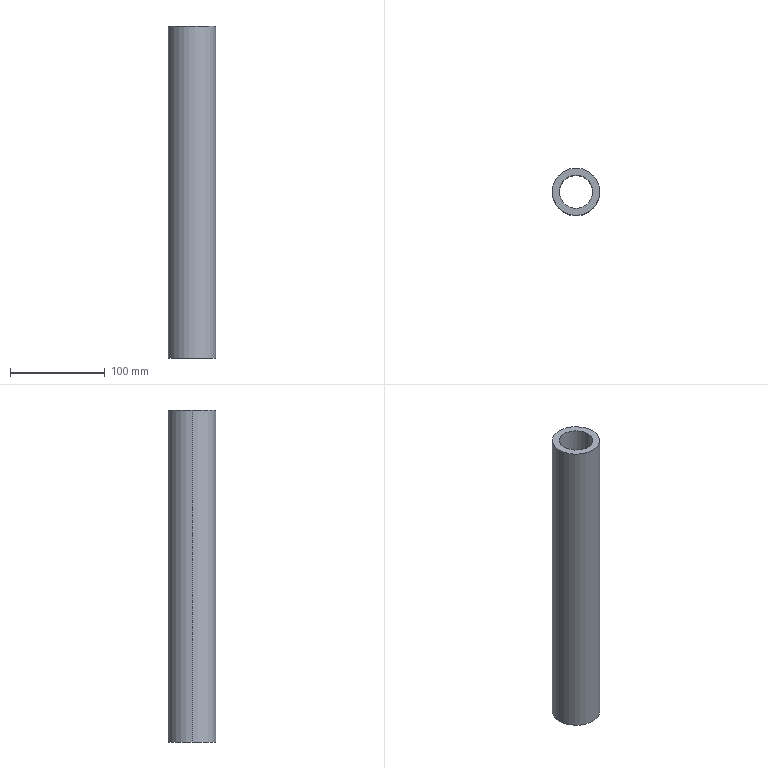Part | STEP file | mounting assembly column ZCD06-D50-L350 | 1 solid | 6 faces | box 50 x 50 x 350 mm | volume 350484 mm3 | cylinder 4 | plane 2 | commonest cylinder face diameters 35 x2 50 x2
STEP:
#1=CARTESIAN_POINT('',(0.,0.,0.));
#2=DIRECTION('',(0.,0.,1.));
#3=DIRECTION('',(1.,0.,0.));
#4=AXIS2_PLACEMENT_3D('',#1,#2,#3);
#5=CARTESIAN_POINT('',(25.,0.,0.));
#6=VERTEX_POINT('',#5);
#7=CARTESIAN_POINT('',(-25.,0.,0.));
#8=VERTEX_POINT('',#7);
#9=CARTESIAN_POINT('',(0.,0.,0.));
#10=DIRECTION('',(0.,0.,1.));
#11=DIRECTION('',(1.,0.,0.));
#12=AXIS2_PLACEMENT_3D('',#9,#10,#11);
#13=CIRCLE('',#12,25.);
#14=CARTESIAN_POINT('',(0.,0.,460.));
#15=DIRECTION('',(0.,0.,1.));
#16=DIRECTION('',(1.,0.,0.));
#17=AXIS2_PLACEMENT_3D('',#14,#15,#16);
#18=CYLINDRICAL_SURFACE('',#17,25.);
#19=CARTESIAN_POINT('',(0.,-460.));
#20=DIRECTION('',(1.,0.));
#21=VECTOR('',#20,1.);
#22=LINE('',#19,#21);
#23=(GEOMETRIC_REPRESENTATION_CONTEXT(2)PARAMETRIC_REPRESENTATION_CONTEXT()REPRESENTATION_CONTEXT('',''));
#24=DEFINITIONAL_REPRESENTATION('',(#22),#23);
#25=PCURVE('',#18,#24);
#26=CARTESIAN_POINT('',(0.,0.,0.));
#27=DIRECTION('',(0.,0.,1.));
#28=DIRECTION('',(1.,0.,0.));
#29=AXIS2_PLACEMENT_3D('',#26,#27,#28);
#30=PLANE('',#29);
#31=CARTESIAN_POINT('',(0.,0.));
#32=DIRECTION('',(1.,0.));
#33=AXIS2_PLACEMENT_2D('',#31,#32);
#34=CIRCLE('',#33,25.);
#35=(GEOMETRIC_REPRESENTATION_CONTEXT(2)PARAMETRIC_REPRESENTATION_CONTEXT()REPRESENTATION_CONTEXT('',''));
#36=DEFINITIONAL_REPRESENTATION('',(#34),#35);
#37=PCURVE('',#30,#36);
#38=SURFACE_CURVE('',#13,(#25,#37),.PCURVE_S1.);
#39=EDGE_CURVE('',#6,#8,#38,.T.);
#40=ORIENTED_EDGE('',*,*,#39,.T.);
#41=CARTESIAN_POINT('',(-25.,0.,350.));
#42=VERTEX_POINT('',#41);
#43=CARTESIAN_POINT('',(-25.,0.,460.));
#44=DIRECTION('',(0.,0.,1.));
#45=VECTOR('',#44,1.);
#46=LINE('',#43,#45);
#47=CARTESIAN_POINT('',(3.142,0.));
#48=DIRECTION('',(0.,1.));
#49=VECTOR('',#48,1.);
#50=LINE('',#47,#49);
#51=(GEOMETRIC_REPRESENTATION_CONTEXT(2)PARAMETRIC_REPRESENTATION_CONTEXT()REPRESENTATION_CONTEXT('',''));
#52=DEFINITIONAL_REPRESENTATION('',(#50),#51);
#53=PCURVE('',#18,#52);
#54=CARTESIAN_POINT('',(0.,0.,460.));
#55=DIRECTION('',(0.,0.,1.));
#56=DIRECTION('',(1.,0.,0.));
#57=AXIS2_PLACEMENT_3D('',#54,#55,#56);
#58=CYLINDRICAL_SURFACE('',#57,25.);
#59=CARTESIAN_POINT('',(3.142,0.));
#60=DIRECTION('',(0.,1.));
#61=VECTOR('',#60,1.);
#62=LINE('',#59,#61);
#63=(GEOMETRIC_REPRESENTATION_CONTEXT(2)PARAMETRIC_REPRESENTATION_CONTEXT()REPRESENTATION_CONTEXT('',''));
#64=DEFINITIONAL_REPRESENTATION('',(#62),#63);
#65=PCURVE('',#58,#64);
#66=SURFACE_CURVE('',#46,(#53,#65),.PCURVE_S1.);
#67=EDGE_CURVE('',#8,#42,#66,.T.);
#68=ORIENTED_EDGE('',*,*,#67,.T.);
#69=CARTESIAN_POINT('',(25.,0.,350.));
#70=VERTEX_POINT('',#69);
#71=CARTESIAN_POINT('',(0.,0.,350.));
#72=DIRECTION('',(0.,0.,1.));
#73=DIRECTION('',(1.,0.,0.));
#74=AXIS2_PLACEMENT_3D('',#71,#72,#73);
#75=CIRCLE('',#74,25.);
#76=CARTESIAN_POINT('',(0.,-110.));
#77=DIRECTION('',(1.,0.));
#78=VECTOR('',#77,1.);
#79=LINE('',#76,#78);
#80=(GEOMETRIC_REPRESENTATION_CONTEXT(2)PARAMETRIC_REPRESENTATION_CONTEXT()REPRESENTATION_CONTEXT('',''));
#81=DEFINITIONAL_REPRESENTATION('',(#79),#80);
#82=PCURVE('',#18,#81);
#83=CARTESIAN_POINT('',(0.,0.,350.));
#84=DIRECTION('',(0.,0.,1.));
#85=DIRECTION('',(1.,0.,0.));
#86=AXIS2_PLACEMENT_3D('',#83,#84,#85);
#87=PLANE('',#86);
#88=CARTESIAN_POINT('',(0.,0.));
#89=DIRECTION('',(1.,0.));
#90=AXIS2_PLACEMENT_2D('',#88,#89);
#91=CIRCLE('',#90,25.);
#92=(GEOMETRIC_REPRESENTATION_CONTEXT(2)PARAMETRIC_REPRESENTATION_CONTEXT()REPRESENTATION_CONTEXT('',''));
#93=DEFINITIONAL_REPRESENTATION('',(#91),#92);
#94=PCURVE('',#87,#93);
#95=SURFACE_CURVE('',#75,(#82,#94),.PCURVE_S1.);
#96=EDGE_CURVE('',#70,#42,#95,.T.);
#97=ORIENTED_EDGE('',*,*,#96,.F.);
#98=CARTESIAN_POINT('',(25.,0.,460.));
#99=DIRECTION('',(0.,0.,1.));
#100=VECTOR('',#99,1.);
#101=LINE('',#98,#100);
#102=CARTESIAN_POINT('',(0.,0.));
#103=DIRECTION('',(0.,1.));
#104=VECTOR('',#103,1.);
#105=LINE('',#102,#104);
#106=(GEOMETRIC_REPRESENTATION_CONTEXT(2)PARAMETRIC_REPRESENTATION_CONTEXT()REPRESENTATION_CONTEXT('',''));
#107=DEFINITIONAL_REPRESENTATION('',(#105),#106);
#108=PCURVE('',#18,#107);
#109=CARTESIAN_POINT('',(6.283,0.));
#110=DIRECTION('',(0.,1.));
#111=VECTOR('',#110,1.);
#112=LINE('',#109,#111);
#113=(GEOMETRIC_REPRESENTATION_CONTEXT(2)PARAMETRIC_REPRESENTATION_CONTEXT()REPRESENTATION_CONTEXT('',''));
#114=DEFINITIONAL_REPRESENTATION('',(#112),#113);
#115=PCURVE('',#58,#114);
#116=SURFACE_CURVE('',#101,(#108,#115),.PCURVE_S1.);
#117=EDGE_CURVE('',#6,#70,#116,.T.);
#118=ORIENTED_EDGE('',*,*,#117,.F.);
#119=EDGE_LOOP('',(#40,#68,#97,#118));
#120=FACE_BOUND('',#119,.T.);
#121=ADVANCED_FACE('',(#120),#18,.T.);
#122=CARTESIAN_POINT('',(17.5,0.,0.));
#123=VERTEX_POINT('',#122);
#124=CARTESIAN_POINT('',(17.5,0.,350.));
#125=VERTEX_POINT('',#124);
#126=CARTESIAN_POINT('',(17.5,0.,460.));
#127=DIRECTION('',(0.,0.,1.));
#128=VECTOR('',#127,1.);
#129=LINE('',#126,#128);
#130=CARTESIAN_POINT('',(0.,0.,460.));
#131=DIRECTION('',(0.,0.,1.));
#132=DIRECTION('',(1.,0.,0.));
#133=AXIS2_PLACEMENT_3D('',#130,#131,#132);
#134=CYLINDRICAL_SURFACE('',#133,17.5);
#135=CARTESIAN_POINT('',(6.283,0.));
#136=DIRECTION('',(0.,1.));
#137=VECTOR('',#136,1.);
#138=LINE('',#135,#137);
#139=(GEOMETRIC_REPRESENTATION_CONTEXT(2)PARAMETRIC_REPRESENTATION_CONTEXT()REPRESENTATION_CONTEXT('',''));
#140=DEFINITIONAL_REPRESENTATION('',(#138),#139);
#141=PCURVE('',#134,#140);
#142=CARTESIAN_POINT('',(0.,0.,460.));
#143=DIRECTION('',(0.,0.,1.));
#144=DIRECTION('',(1.,0.,0.));
#145=AXIS2_PLACEMENT_3D('',#142,#143,#144);
#146=CYLINDRICAL_SURFACE('',#145,17.5);
#147=CARTESIAN_POINT('',(0.,0.));
#148=DIRECTION('',(0.,1.));
#149=VECTOR('',#148,1.);
#150=LINE('',#147,#149);
#151=(GEOMETRIC_REPRESENTATION_CONTEXT(2)PARAMETRIC_REPRESENTATION_CONTEXT()REPRESENTATION_CONTEXT('',''));
#152=DEFINITIONAL_REPRESENTATION('',(#150),#151);
#153=PCURVE('',#146,#152);
#154=SURFACE_CURVE('',#129,(#141,#153),.PCURVE_S1.);
#155=EDGE_CURVE('',#123,#125,#154,.T.);
#156=ORIENTED_EDGE('',*,*,#155,.T.);
#157=CARTESIAN_POINT('',(-17.5,0.,350.));
#158=VERTEX_POINT('',#157);
#159=CARTESIAN_POINT('',(0.,0.,350.));
#160=DIRECTION('',(0.,0.,1.));
#161=DIRECTION('',(1.,0.,0.));
#162=AXIS2_PLACEMENT_3D('',#159,#160,#161);
#163=CIRCLE('',#162,17.5);
#164=CARTESIAN_POINT('',(0.,-110.));
#165=DIRECTION('',(1.,0.));
#166=VECTOR('',#165,1.);
#167=LINE('',#164,#166);
#168=(GEOMETRIC_REPRESENTATION_CONTEXT(2)PARAMETRIC_REPRESENTATION_CONTEXT()REPRESENTATION_CONTEXT('',''));
#169=DEFINITIONAL_REPRESENTATION('',(#167),#168);
#170=PCURVE('',#134,#169);
#171=CARTESIAN_POINT('',(0.,0.));
#172=DIRECTION('',(1.,0.));
#173=AXIS2_PLACEMENT_2D('',#171,#172);
#174=CIRCLE('',#173,17.5);
#175=(GEOMETRIC_REPRESENTATION_CONTEXT(2)PARAMETRIC_REPRESENTATION_CONTEXT()REPRESENTATION_CONTEXT('',''));
#176=DEFINITIONAL_REPRESENTATION('',(#174),#175);
#177=PCURVE('',#87,#176);
#178=SURFACE_CURVE('',#163,(#170,#177),.PCURVE_S1.);
#179=EDGE_CURVE('',#158,#125,#178,.T.);
#180=ORIENTED_EDGE('',*,*,#179,.F.);
#181=CARTESIAN_POINT('',(-17.5,0.,0.));
#182=VERTEX_POINT('',#181);
#183=CARTESIAN_POINT('',(-17.5,0.,460.));
#184=DIRECTION('',(0.,0.,1.));
#185=VECTOR('',#184,1.);
#186=LINE('',#183,#185);
#187=CARTESIAN_POINT('',(3.142,0.));
#188=DIRECTION('',(0.,1.));
#189=VECTOR('',#188,1.);
#190=LINE('',#187,#189);
#191=(GEOMETRIC_REPRESENTATION_CONTEXT(2)PARAMETRIC_REPRESENTATION_CONTEXT()REPRESENTATION_CONTEXT('',''));
#192=DEFINITIONAL_REPRESENTATION('',(#190),#191);
#193=PCURVE('',#134,#192);
#194=CARTESIAN_POINT('',(3.142,0.));
#195=DIRECTION('',(0.,1.));
#196=VECTOR('',#195,1.);
#197=LINE('',#194,#196);
#198=(GEOMETRIC_REPRESENTATION_CONTEXT(2)PARAMETRIC_REPRESENTATION_CONTEXT()REPRESENTATION_CONTEXT('',''));
#199=DEFINITIONAL_REPRESENTATION('',(#197),#198);
#200=PCURVE('',#146,#199);
#201=SURFACE_CURVE('',#186,(#193,#200),.PCURVE_S1.);
#202=EDGE_CURVE('',#182,#158,#201,.T.);
#203=ORIENTED_EDGE('',*,*,#202,.F.);
#204=CARTESIAN_POINT('',(0.,0.,0.));
#205=DIRECTION('',(0.,0.,-1.));
#206=DIRECTION('',(1.,0.,0.));
#207=AXIS2_PLACEMENT_3D('',#204,#205,#206);
#208=CIRCLE('',#207,17.5);
#209=CARTESIAN_POINT('',(6.283,-460.));
#210=DIRECTION('',(-1.,0.));
#211=VECTOR('',#210,1.);
#212=LINE('',#209,#211);
#213=(GEOMETRIC_REPRESENTATION_CONTEXT(2)PARAMETRIC_REPRESENTATION_CONTEXT()REPRESENTATION_CONTEXT('',''));
#214=DEFINITIONAL_REPRESENTATION('',(#212),#213);
#215=PCURVE('',#134,#214);
#216=CARTESIAN_POINT('',(17.5,0.));
#217=CARTESIAN_POINT('',(17.5,-30.311));
#218=CARTESIAN_POINT('',(-8.75,-15.155));
#219=CARTESIAN_POINT('',(-35.,0.));
#220=CARTESIAN_POINT('',(-8.75,15.155));
#221=CARTESIAN_POINT('',(17.5,30.311));
#222=CARTESIAN_POINT('',(17.5,0.));
#223=(BOUNDED_CURVE()B_SPLINE_CURVE(2,(#216,#217,#218,#219,#220,#221,#222),.UNSPECIFIED.,.T.,.F.)B_SPLINE_CURVE_WITH_KNOTS((1,2,2,2,2,1),(-2.094,0.,2.094,4.189,6.283,8.378),.UNSPECIFIED.)CURVE()GEOMETRIC_REPRESENTATION_ITEM()RATIONAL_B_SPLINE_CURVE((1.,0.5,1.,0.5,1.,0.5,1.))REPRESENTATION_ITEM(''));
#224=(GEOMETRIC_REPRESENTATION_CONTEXT(2)PARAMETRIC_REPRESENTATION_CONTEXT()REPRESENTATION_CONTEXT('',''));
#225=DEFINITIONAL_REPRESENTATION('',(#223),#224);
#226=PCURVE('',#30,#225);
#227=SURFACE_CURVE('',#208,(#215,#226),.PCURVE_S1.);
#228=EDGE_CURVE('',#123,#182,#227,.T.);
#229=ORIENTED_EDGE('',*,*,#228,.F.);
#230=EDGE_LOOP('',(#156,#180,#203,#229));
#231=FACE_BOUND('',#230,.F.);
#232=ADVANCED_FACE('',(#231),#134,.F.);
#233=ORIENTED_EDGE('',*,*,#67,.F.);
#234=CARTESIAN_POINT('',(0.,0.,0.));
#235=DIRECTION('',(0.,0.,1.));
#236=DIRECTION('',(1.,0.,0.));
#237=AXIS2_PLACEMENT_3D('',#234,#235,#236);
#238=CIRCLE('',#237,25.);
#239=CARTESIAN_POINT('',(0.,-460.));
#240=DIRECTION('',(1.,0.));
#241=VECTOR('',#240,1.);
#242=LINE('',#239,#241);
#243=(GEOMETRIC_REPRESENTATION_CONTEXT(2)PARAMETRIC_REPRESENTATION_CONTEXT()REPRESENTATION_CONTEXT('',''));
#244=DEFINITIONAL_REPRESENTATION('',(#242),#243);
#245=PCURVE('',#58,#244);
#246=CARTESIAN_POINT('',(0.,0.));
#247=DIRECTION('',(1.,0.));
#248=AXIS2_PLACEMENT_2D('',#246,#247);
#249=CIRCLE('',#248,25.);
#250=(GEOMETRIC_REPRESENTATION_CONTEXT(2)PARAMETRIC_REPRESENTATION_CONTEXT()REPRESENTATION_CONTEXT('',''));
#251=DEFINITIONAL_REPRESENTATION('',(#249),#250);
#252=PCURVE('',#30,#251);
#253=SURFACE_CURVE('',#238,(#245,#252),.PCURVE_S1.);
#254=EDGE_CURVE('',#8,#6,#253,.T.);
#255=ORIENTED_EDGE('',*,*,#254,.T.);
#256=ORIENTED_EDGE('',*,*,#117,.T.);
#257=CARTESIAN_POINT('',(0.,0.,350.));
#258=DIRECTION('',(0.,0.,1.));
#259=DIRECTION('',(1.,0.,0.));
#260=AXIS2_PLACEMENT_3D('',#257,#258,#259);
#261=CIRCLE('',#260,25.);
#262=CARTESIAN_POINT('',(0.,-110.));
#263=DIRECTION('',(1.,0.));
#264=VECTOR('',#263,1.);
#265=LINE('',#262,#264);
#266=(GEOMETRIC_REPRESENTATION_CONTEXT(2)PARAMETRIC_REPRESENTATION_CONTEXT()REPRESENTATION_CONTEXT('',''));
#267=DEFINITIONAL_REPRESENTATION('',(#265),#266);
#268=PCURVE('',#58,#267);
#269=CARTESIAN_POINT('',(0.,0.));
#270=DIRECTION('',(1.,0.));
#271=AXIS2_PLACEMENT_2D('',#269,#270);
#272=CIRCLE('',#271,25.);
#273=(GEOMETRIC_REPRESENTATION_CONTEXT(2)PARAMETRIC_REPRESENTATION_CONTEXT()REPRESENTATION_CONTEXT('',''));
#274=DEFINITIONAL_REPRESENTATION('',(#272),#273);
#275=PCURVE('',#87,#274);
#276=SURFACE_CURVE('',#261,(#268,#275),.PCURVE_S1.);
#277=EDGE_CURVE('',#42,#70,#276,.T.);
#278=ORIENTED_EDGE('',*,*,#277,.F.);
#279=EDGE_LOOP('',(#233,#255,#256,#278));
#280=FACE_BOUND('',#279,.T.);
#281=ADVANCED_FACE('',(#280),#58,.T.);
#282=ORIENTED_EDGE('',*,*,#39,.F.);
#283=ORIENTED_EDGE('',*,*,#254,.F.);
#284=EDGE_LOOP('',(#282,#283));
#285=FACE_BOUND('',#284,.T.);
#286=ORIENTED_EDGE('',*,*,#228,.F.);
#287=CARTESIAN_POINT('',(0.,0.,0.));
#288=DIRECTION('',(0.,0.,-1.));
#289=DIRECTION('',(1.,0.,0.));
#290=AXIS2_PLACEMENT_3D('',#287,#288,#289);
#291=CIRCLE('',#290,17.5);
#292=CARTESIAN_POINT('',(17.5,0.));
#293=CARTESIAN_POINT('',(17.5,-30.311));
#294=CARTESIAN_POINT('',(-8.75,-15.155));
#295=CARTESIAN_POINT('',(-35.,0.));
#296=CARTESIAN_POINT('',(-8.75,15.155));
#297=CARTESIAN_POINT('',(17.5,30.311));
#298=CARTESIAN_POINT('',(17.5,0.));
#299=(BOUNDED_CURVE()B_SPLINE_CURVE(2,(#292,#293,#294,#295,#296,#297,#298),.UNSPECIFIED.,.T.,.F.)B_SPLINE_CURVE_WITH_KNOTS((1,2,2,2,2,1),(-2.094,0.,2.094,4.189,6.283,8.378),.UNSPECIFIED.)CURVE()GEOMETRIC_REPRESENTATION_ITEM()RATIONAL_B_SPLINE_CURVE((1.,0.5,1.,0.5,1.,0.5,1.))REPRESENTATION_ITEM(''));
#300=(GEOMETRIC_REPRESENTATION_CONTEXT(2)PARAMETRIC_REPRESENTATION_CONTEXT()REPRESENTATION_CONTEXT('',''));
#301=DEFINITIONAL_REPRESENTATION('',(#299),#300);
#302=PCURVE('',#30,#301);
#303=CARTESIAN_POINT('',(6.283,-460.));
#304=DIRECTION('',(-1.,0.));
#305=VECTOR('',#304,1.);
#306=LINE('',#303,#305);
#307=(GEOMETRIC_REPRESENTATION_CONTEXT(2)PARAMETRIC_REPRESENTATION_CONTEXT()REPRESENTATION_CONTEXT('',''));
#308=DEFINITIONAL_REPRESENTATION('',(#306),#307);
#309=PCURVE('',#146,#308);
#310=SURFACE_CURVE('',#291,(#302,#309),.PCURVE_S1.);
#311=EDGE_CURVE('',#182,#123,#310,.T.);
#312=ORIENTED_EDGE('',*,*,#311,.F.);
#313=EDGE_LOOP('',(#286,#312));
#314=FACE_BOUND('',#313,.T.);
#315=ADVANCED_FACE('',(#285,#314),#30,.F.);
#316=CARTESIAN_POINT('',(0.,0.,350.));
#317=DIRECTION('',(0.,0.,1.));
#318=DIRECTION('',(1.,0.,0.));
#319=AXIS2_PLACEMENT_3D('',#316,#317,#318);
#320=CIRCLE('',#319,17.5);
#321=CARTESIAN_POINT('',(0.,-110.));
#322=DIRECTION('',(1.,0.));
#323=VECTOR('',#322,1.);
#324=LINE('',#321,#323);
#325=(GEOMETRIC_REPRESENTATION_CONTEXT(2)PARAMETRIC_REPRESENTATION_CONTEXT()REPRESENTATION_CONTEXT('',''));
#326=DEFINITIONAL_REPRESENTATION('',(#324),#325);
#327=PCURVE('',#146,#326);
#328=CARTESIAN_POINT('',(0.,0.));
#329=DIRECTION('',(1.,0.));
#330=AXIS2_PLACEMENT_2D('',#328,#329);
#331=CIRCLE('',#330,17.5);
#332=(GEOMETRIC_REPRESENTATION_CONTEXT(2)PARAMETRIC_REPRESENTATION_CONTEXT()REPRESENTATION_CONTEXT('',''));
#333=DEFINITIONAL_REPRESENTATION('',(#331),#332);
#334=PCURVE('',#87,#333);
#335=SURFACE_CURVE('',#320,(#327,#334),.PCURVE_S1.);
#336=EDGE_CURVE('',#125,#158,#335,.T.);
#337=ORIENTED_EDGE('',*,*,#336,.F.);
#338=ORIENTED_EDGE('',*,*,#155,.F.);
#339=ORIENTED_EDGE('',*,*,#311,.F.);
#340=ORIENTED_EDGE('',*,*,#202,.T.);
#341=EDGE_LOOP('',(#337,#338,#339,#340));
#342=FACE_BOUND('',#341,.F.);
#343=ADVANCED_FACE('',(#342),#146,.F.);
#344=ORIENTED_EDGE('',*,*,#96,.T.);
#345=ORIENTED_EDGE('',*,*,#277,.T.);
#346=EDGE_LOOP('',(#344,#345));
#347=FACE_BOUND('',#346,.T.);
#348=ORIENTED_EDGE('',*,*,#336,.F.);
#349=ORIENTED_EDGE('',*,*,#179,.F.);
#350=EDGE_LOOP('',(#348,#349));
#351=FACE_BOUND('',#350,.T.);
#352=ADVANCED_FACE('',(#347,#351),#87,.T.);
#353=CLOSED_SHELL('',(#121,#232,#281,#315,#343,#352));
#354=MANIFOLD_SOLID_BREP('',#353);
#355=(LENGTH_UNIT()NAMED_UNIT(*)SI_UNIT(.MILLI.,.METRE.));
#356=UNCERTAINTY_MEASURE_WITH_UNIT(LENGTH_MEASURE(0.0000001),#355,'','');
#357=(NAMED_UNIT(*)PLANE_ANGLE_UNIT()SI_UNIT($,.RADIAN.));
#358=(NAMED_UNIT(*)SI_UNIT($,.STERADIAN.)SOLID_ANGLE_UNIT());
#359=(GEOMETRIC_REPRESENTATION_CONTEXT(3)GLOBAL_UNCERTAINTY_ASSIGNED_CONTEXT((#356))GLOBAL_UNIT_ASSIGNED_CONTEXT((#355,#357,#358))REPRESENTATION_CONTEXT('',''));
#360=ADVANCED_BREP_SHAPE_REPRESENTATION('',(#4,#354),#359);